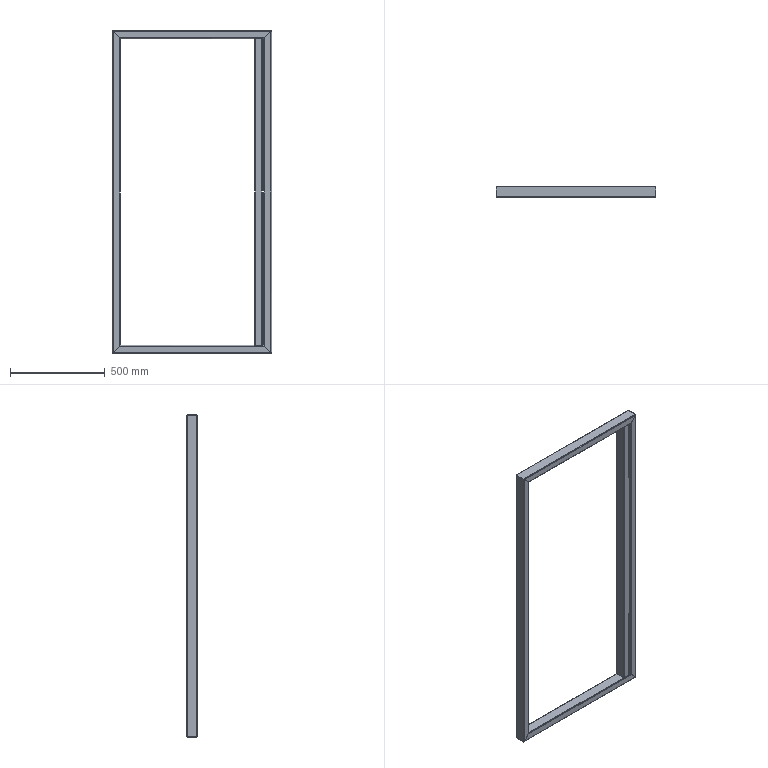Part | STEP file | Base_Default<Machined> | 5 solids | 90 faces | box 840 x 60 x 1700 mm | volume 2443992 mm3 | plane 50 | cylinder 40 | commonest cylinder face diameters 4 x20 8 x20